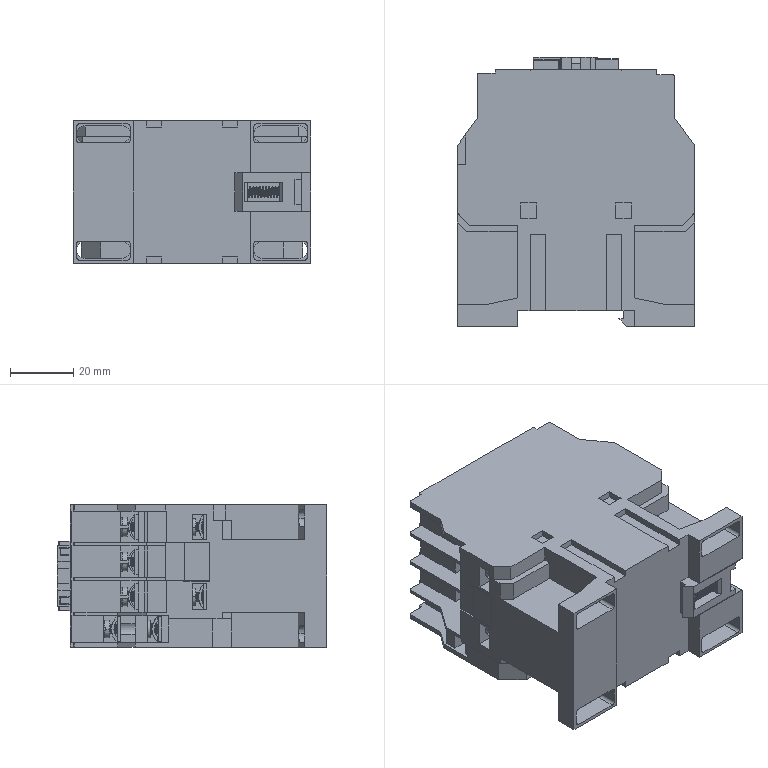Part | STEP file | contactor NXC-12 | 25 solids | 1694 faces | box 75 x 85 x 45 mm | volume 200816 mm3 | plane 1131 | cylinder 463 | spline 57 | torus 34 | sphere 9 | commonest cylinder face diameters 3 x216 0.4 x57 2 x34 5.5 x28 6.5 x24 3.5 x22